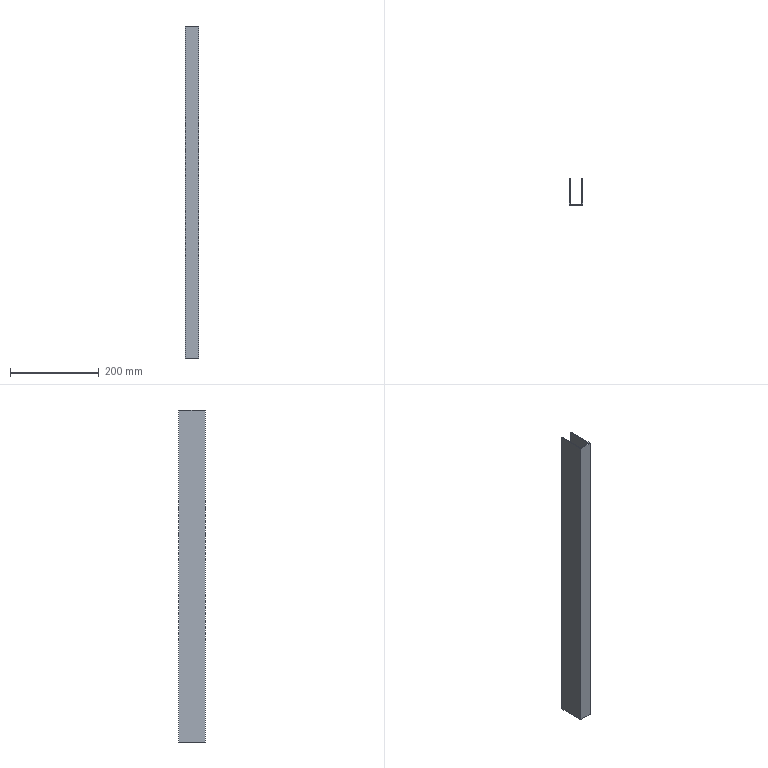Part | SolidWorks | features Extrusion 1, Shell 1 | 1 solid | 10 faces | box 30 x 60 x 748 mm | volume 218416 mm3 | plane 10
STEP:
#1=CARTESIAN_POINT('',(13.,30.,374.));
#2=VERTEX_POINT('',#1);
#3=CARTESIAN_POINT('',(13.,30.,-374.));
#4=VERTEX_POINT('',#3);
#5=CARTESIAN_POINT('',(13.,30.,374.));
#6=DIRECTION('',(0.,0.,-1.));
#7=VECTOR('',#6,1000.);
#8=LINE('',#5,#7);
#9=EDGE_CURVE('',#2,#4,#8,.T.);
#10=ORIENTED_EDGE('',*,*,#9,.F.);
#11=CARTESIAN_POINT('',(15.,30.,374.));
#12=VERTEX_POINT('',#11);
#13=CARTESIAN_POINT('',(-15.,30.,374.));
#14=DIRECTION('',(-1.,0.,0.));
#15=VECTOR('',#14,1000.);
#16=LINE('',#13,#15);
#17=EDGE_CURVE('',#12,#2,#16,.T.);
#18=ORIENTED_EDGE('',*,*,#17,.F.);
#19=CARTESIAN_POINT('',(15.,30.,-374.));
#20=VERTEX_POINT('',#19);
#21=CARTESIAN_POINT('',(15.,30.,374.));
#22=DIRECTION('',(0.,0.,-1.));
#23=VECTOR('',#22,1000.);
#24=LINE('',#21,#23);
#25=EDGE_CURVE('',#12,#20,#24,.T.);
#26=ORIENTED_EDGE('',*,*,#25,.T.);
#27=CARTESIAN_POINT('',(-15.,30.,-374.));
#28=DIRECTION('',(-1.,0.,0.));
#29=VECTOR('',#28,1000.);
#30=LINE('',#27,#29);
#31=EDGE_CURVE('',#20,#4,#30,.T.);
#32=ORIENTED_EDGE('',*,*,#31,.T.);
#33=EDGE_LOOP('',(#10,#18,#26,#32));
#34=FACE_OUTER_BOUND('',#33,.T.);
#35=CARTESIAN_POINT('',(-15.,30.,374.));
#36=DIRECTION('',(0.,-1.,0.));
#37=DIRECTION('',(0.,0.,-1.));
#38=AXIS2_PLACEMENT_3D('',#35,#36,#37);
#39=PLANE('',#38);
#40=ADVANCED_FACE('',(#34),#39,.F.);
#41=CARTESIAN_POINT('',(13.,-28.,374.));
#42=VERTEX_POINT('',#41);
#43=CARTESIAN_POINT('',(13.,0.,374.));
#44=DIRECTION('',(0.,1.,0.));
#45=VECTOR('',#44,1000.);
#46=LINE('',#43,#45);
#47=EDGE_CURVE('',#42,#2,#46,.T.);
#48=ORIENTED_EDGE('',*,*,#47,.F.);
#49=CARTESIAN_POINT('',(-13.,-28.,374.));
#50=VERTEX_POINT('',#49);
#51=CARTESIAN_POINT('',(0.,-28.,374.));
#52=DIRECTION('',(1.,0.,0.));
#53=VECTOR('',#52,1000.);
#54=LINE('',#51,#53);
#55=EDGE_CURVE('',#50,#42,#54,.T.);
#56=ORIENTED_EDGE('',*,*,#55,.F.);
#57=CARTESIAN_POINT('',(-13.,30.,374.));
#58=VERTEX_POINT('',#57);
#59=CARTESIAN_POINT('',(-13.,0.,374.));
#60=DIRECTION('',(0.,-1.,0.));
#61=VECTOR('',#60,1000.);
#62=LINE('',#59,#61);
#63=EDGE_CURVE('',#58,#50,#62,.T.);
#64=ORIENTED_EDGE('',*,*,#63,.F.);
#65=CARTESIAN_POINT('',(-15.,30.,374.));
#66=VERTEX_POINT('',#65);
#67=CARTESIAN_POINT('',(-15.,30.,374.));
#68=DIRECTION('',(-1.,0.,0.));
#69=VECTOR('',#68,1000.);
#70=LINE('',#67,#69);
#71=EDGE_CURVE('',#58,#66,#70,.T.);
#72=ORIENTED_EDGE('',*,*,#71,.T.);
#73=CARTESIAN_POINT('',(-15.,-30.,374.));
#74=VERTEX_POINT('',#73);
#75=CARTESIAN_POINT('',(-15.,-30.,374.));
#76=DIRECTION('',(0.,-1.,0.));
#77=VECTOR('',#76,1000.);
#78=LINE('',#75,#77);
#79=EDGE_CURVE('',#66,#74,#78,.T.);
#80=ORIENTED_EDGE('',*,*,#79,.T.);
#81=CARTESIAN_POINT('',(15.,-30.,374.));
#82=VERTEX_POINT('',#81);
#83=CARTESIAN_POINT('',(-15.,-30.,374.));
#84=DIRECTION('',(1.,0.,0.));
#85=VECTOR('',#84,1000.);
#86=LINE('',#83,#85);
#87=EDGE_CURVE('',#74,#82,#86,.T.);
#88=ORIENTED_EDGE('',*,*,#87,.T.);
#89=CARTESIAN_POINT('',(15.,-30.,374.));
#90=DIRECTION('',(0.,1.,0.));
#91=VECTOR('',#90,1000.);
#92=LINE('',#89,#91);
#93=EDGE_CURVE('',#82,#12,#92,.T.);
#94=ORIENTED_EDGE('',*,*,#93,.T.);
#95=ORIENTED_EDGE('',*,*,#17,.T.);
#96=EDGE_LOOP('',(#48,#56,#64,#72,#80,#88,#94,#95));
#97=FACE_OUTER_BOUND('',#96,.T.);
#98=CARTESIAN_POINT('',(0.,0.,374.));
#99=DIRECTION('',(0.,0.,-1.));
#100=DIRECTION('',(-1.,0.,0.));
#101=AXIS2_PLACEMENT_3D('',#98,#99,#100);
#102=PLANE('',#101);
#103=ADVANCED_FACE('',(#97),#102,.F.);
#104=CARTESIAN_POINT('',(-13.,-28.,-374.));
#105=VERTEX_POINT('',#104);
#106=CARTESIAN_POINT('',(13.,-28.,-374.));
#107=VERTEX_POINT('',#106);
#108=CARTESIAN_POINT('',(0.,-28.,-374.));
#109=DIRECTION('',(1.,0.,0.));
#110=VECTOR('',#109,1000.);
#111=LINE('',#108,#110);
#112=EDGE_CURVE('',#105,#107,#111,.T.);
#113=ORIENTED_EDGE('',*,*,#112,.T.);
#114=CARTESIAN_POINT('',(13.,0.,-374.));
#115=DIRECTION('',(0.,1.,0.));
#116=VECTOR('',#115,1000.);
#117=LINE('',#114,#116);
#118=EDGE_CURVE('',#107,#4,#117,.T.);
#119=ORIENTED_EDGE('',*,*,#118,.T.);
#120=ORIENTED_EDGE('',*,*,#31,.F.);
#121=CARTESIAN_POINT('',(15.,-30.,-374.));
#122=VERTEX_POINT('',#121);
#123=CARTESIAN_POINT('',(15.,-30.,-374.));
#124=DIRECTION('',(0.,1.,0.));
#125=VECTOR('',#124,1000.);
#126=LINE('',#123,#125);
#127=EDGE_CURVE('',#122,#20,#126,.T.);
#128=ORIENTED_EDGE('',*,*,#127,.F.);
#129=CARTESIAN_POINT('',(-15.,-30.,-374.));
#130=VERTEX_POINT('',#129);
#131=CARTESIAN_POINT('',(-15.,-30.,-374.));
#132=DIRECTION('',(1.,0.,0.));
#133=VECTOR('',#132,1000.);
#134=LINE('',#131,#133);
#135=EDGE_CURVE('',#130,#122,#134,.T.);
#136=ORIENTED_EDGE('',*,*,#135,.F.);
#137=CARTESIAN_POINT('',(-15.,30.,-374.));
#138=VERTEX_POINT('',#137);
#139=CARTESIAN_POINT('',(-15.,-30.,-374.));
#140=DIRECTION('',(0.,-1.,0.));
#141=VECTOR('',#140,1000.);
#142=LINE('',#139,#141);
#143=EDGE_CURVE('',#138,#130,#142,.T.);
#144=ORIENTED_EDGE('',*,*,#143,.F.);
#145=CARTESIAN_POINT('',(-13.,30.,-374.));
#146=VERTEX_POINT('',#145);
#147=CARTESIAN_POINT('',(-15.,30.,-374.));
#148=DIRECTION('',(-1.,0.,0.));
#149=VECTOR('',#148,1000.);
#150=LINE('',#147,#149);
#151=EDGE_CURVE('',#146,#138,#150,.T.);
#152=ORIENTED_EDGE('',*,*,#151,.F.);
#153=CARTESIAN_POINT('',(-13.,0.,-374.));
#154=DIRECTION('',(0.,-1.,0.));
#155=VECTOR('',#154,1000.);
#156=LINE('',#153,#155);
#157=EDGE_CURVE('',#146,#105,#156,.T.);
#158=ORIENTED_EDGE('',*,*,#157,.T.);
#159=EDGE_LOOP('',(#113,#119,#120,#128,#136,#144,#152,#158));
#160=FACE_OUTER_BOUND('',#159,.T.);
#161=CARTESIAN_POINT('',(0.,0.,-374.));
#162=DIRECTION('',(0.,0.,-1.));
#163=DIRECTION('',(-1.,0.,0.));
#164=AXIS2_PLACEMENT_3D('',#161,#162,#163);
#165=PLANE('',#164);
#166=ADVANCED_FACE('',(#160),#165,.T.);
#167=ORIENTED_EDGE('',*,*,#127,.T.);
#168=ORIENTED_EDGE('',*,*,#25,.F.);
#169=ORIENTED_EDGE('',*,*,#93,.F.);
#170=CARTESIAN_POINT('',(15.,-30.,374.));
#171=DIRECTION('',(0.,0.,-1.));
#172=VECTOR('',#171,1000.);
#173=LINE('',#170,#172);
#174=EDGE_CURVE('',#82,#122,#173,.T.);
#175=ORIENTED_EDGE('',*,*,#174,.T.);
#176=EDGE_LOOP('',(#167,#168,#169,#175));
#177=FACE_OUTER_BOUND('',#176,.T.);
#178=CARTESIAN_POINT('',(15.,-30.,374.));
#179=DIRECTION('',(-1.,0.,0.));
#180=DIRECTION('',(0.,0.,1.));
#181=AXIS2_PLACEMENT_3D('',#178,#179,#180);
#182=PLANE('',#181);
#183=ADVANCED_FACE('',(#177),#182,.F.);
#184=ORIENTED_EDGE('',*,*,#71,.F.);
#185=CARTESIAN_POINT('',(-13.,30.,374.));
#186=DIRECTION('',(0.,0.,-1.));
#187=VECTOR('',#186,1000.);
#188=LINE('',#185,#187);
#189=EDGE_CURVE('',#58,#146,#188,.T.);
#190=ORIENTED_EDGE('',*,*,#189,.T.);
#191=ORIENTED_EDGE('',*,*,#151,.T.);
#192=CARTESIAN_POINT('',(-15.,30.,374.));
#193=DIRECTION('',(0.,0.,-1.));
#194=VECTOR('',#193,1000.);
#195=LINE('',#192,#194);
#196=EDGE_CURVE('',#66,#138,#195,.T.);
#197=ORIENTED_EDGE('',*,*,#196,.F.);
#198=EDGE_LOOP('',(#184,#190,#191,#197));
#199=FACE_OUTER_BOUND('',#198,.T.);
#200=CARTESIAN_POINT('',(-15.,30.,374.));
#201=DIRECTION('',(0.,-1.,0.));
#202=DIRECTION('',(0.,0.,-1.));
#203=AXIS2_PLACEMENT_3D('',#200,#201,#202);
#204=PLANE('',#203);
#205=ADVANCED_FACE('',(#199),#204,.F.);
#206=ORIENTED_EDGE('',*,*,#143,.T.);
#207=CARTESIAN_POINT('',(-15.,-30.,374.));
#208=DIRECTION('',(0.,0.,-1.));
#209=VECTOR('',#208,1000.);
#210=LINE('',#207,#209);
#211=EDGE_CURVE('',#74,#130,#210,.T.);
#212=ORIENTED_EDGE('',*,*,#211,.F.);
#213=ORIENTED_EDGE('',*,*,#79,.F.);
#214=ORIENTED_EDGE('',*,*,#196,.T.);
#215=EDGE_LOOP('',(#206,#212,#213,#214));
#216=FACE_OUTER_BOUND('',#215,.T.);
#217=CARTESIAN_POINT('',(-15.,-30.,374.));
#218=DIRECTION('',(1.,0.,0.));
#219=DIRECTION('',(0.,0.,-1.));
#220=AXIS2_PLACEMENT_3D('',#217,#218,#219);
#221=PLANE('',#220);
#222=ADVANCED_FACE('',(#216),#221,.F.);
#223=ORIENTED_EDGE('',*,*,#135,.T.);
#224=ORIENTED_EDGE('',*,*,#174,.F.);
#225=ORIENTED_EDGE('',*,*,#87,.F.);
#226=ORIENTED_EDGE('',*,*,#211,.T.);
#227=EDGE_LOOP('',(#223,#224,#225,#226));
#228=FACE_OUTER_BOUND('',#227,.T.);
#229=CARTESIAN_POINT('',(-15.,-30.,374.));
#230=DIRECTION('',(0.,1.,0.));
#231=DIRECTION('',(0.,0.,1.));
#232=AXIS2_PLACEMENT_3D('',#229,#230,#231);
#233=PLANE('',#232);
#234=ADVANCED_FACE('',(#228),#233,.F.);
#235=ORIENTED_EDGE('',*,*,#118,.F.);
#236=CARTESIAN_POINT('',(13.,-28.,374.));
#237=DIRECTION('',(0.,0.,-1.));
#238=VECTOR('',#237,1000.);
#239=LINE('',#236,#238);
#240=EDGE_CURVE('',#42,#107,#239,.T.);
#241=ORIENTED_EDGE('',*,*,#240,.F.);
#242=ORIENTED_EDGE('',*,*,#47,.T.);
#243=ORIENTED_EDGE('',*,*,#9,.T.);
#244=EDGE_LOOP('',(#235,#241,#242,#243));
#245=FACE_OUTER_BOUND('',#244,.T.);
#246=CARTESIAN_POINT('',(13.,-30.,374.));
#247=DIRECTION('',(-1.,0.,0.));
#248=DIRECTION('',(0.,0.,1.));
#249=AXIS2_PLACEMENT_3D('',#246,#247,#248);
#250=PLANE('',#249);
#251=ADVANCED_FACE('',(#245),#250,.T.);
#252=ORIENTED_EDGE('',*,*,#157,.F.);
#253=ORIENTED_EDGE('',*,*,#189,.F.);
#254=ORIENTED_EDGE('',*,*,#63,.T.);
#255=CARTESIAN_POINT('',(-13.,-28.,374.));
#256=DIRECTION('',(0.,0.,-1.));
#257=VECTOR('',#256,1000.);
#258=LINE('',#255,#257);
#259=EDGE_CURVE('',#50,#105,#258,.T.);
#260=ORIENTED_EDGE('',*,*,#259,.T.);
#261=EDGE_LOOP('',(#252,#253,#254,#260));
#262=FACE_OUTER_BOUND('',#261,.T.);
#263=CARTESIAN_POINT('',(-13.,-30.,374.));
#264=DIRECTION('',(1.,0.,0.));
#265=DIRECTION('',(0.,0.,-1.));
#266=AXIS2_PLACEMENT_3D('',#263,#264,#265);
#267=PLANE('',#266);
#268=ADVANCED_FACE('',(#262),#267,.T.);
#269=ORIENTED_EDGE('',*,*,#112,.F.);
#270=ORIENTED_EDGE('',*,*,#259,.F.);
#271=ORIENTED_EDGE('',*,*,#55,.T.);
#272=ORIENTED_EDGE('',*,*,#240,.T.);
#273=EDGE_LOOP('',(#269,#270,#271,#272));
#274=FACE_OUTER_BOUND('',#273,.T.);
#275=CARTESIAN_POINT('',(-15.,-28.,374.));
#276=DIRECTION('',(0.,1.,0.));
#277=DIRECTION('',(0.,0.,1.));
#278=AXIS2_PLACEMENT_3D('',#275,#276,#277);
#279=PLANE('',#278);
#280=ADVANCED_FACE('',(#274),#279,.T.);
#281=CLOSED_SHELL('',(#40,#103,#166,#183,#205,#222,#234,#251,#268,#280));
#282=MANIFOLD_SOLID_BREP('',#281);
#283=CARTESIAN_POINT('',(0.,0.,0.));
#284=DIRECTION('',(0.,0.,1.));
#285=DIRECTION('',(1.,0.,0.));
#286=AXIS2_PLACEMENT_3D('',#283,#284,#285);
#287=(LENGTH_UNIT()NAMED_UNIT(*)SI_UNIT(.MILLI.,.METRE.));
#288=UNCERTAINTY_MEASURE_WITH_UNIT(LENGTH_MEASURE(0.00001),#287,'','');
#289=(NAMED_UNIT(*)PLANE_ANGLE_UNIT()SI_UNIT($,.RADIAN.));
#290=(NAMED_UNIT(*)SI_UNIT($,.STERADIAN.)SOLID_ANGLE_UNIT());
#291=(GEOMETRIC_REPRESENTATION_CONTEXT(3)GLOBAL_UNCERTAINTY_ASSIGNED_CONTEXT((#288))GLOBAL_UNIT_ASSIGNED_CONTEXT((#287,#289,#290))REPRESENTATION_CONTEXT('',''));
#292=ADVANCED_BREP_SHAPE_REPRESENTATION('',(#282,#286),#291);